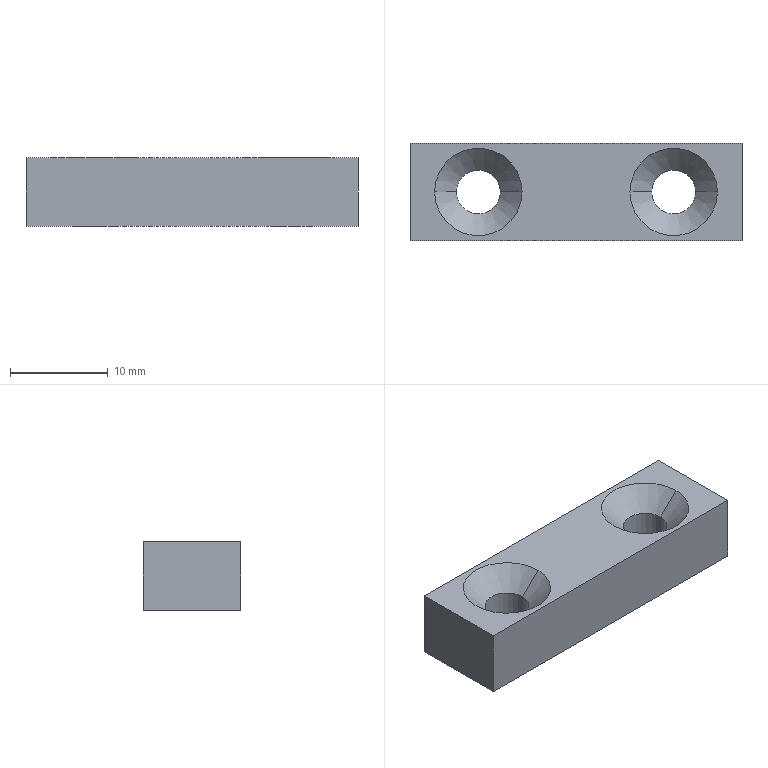Part | STEP file | anti-collision silicone pad | 1 solid | 14 faces | box 34 x 10 x 7 mm | volume 2064 mm3 | plane 6 | cone 4 | cylinder 4 | commonest cylinder face diameters 4.5 x4
STEP:
#1=CARTESIAN_POINT('',(0.,0.,0.));
#2=DIRECTION('',(0.,0.,1.));
#3=DIRECTION('',(1.,0.,0.));
#4=AXIS2_PLACEMENT_3D('',#1,#2,#3);
#5=CARTESIAN_POINT('',(-7.75,0.,4.77));
#6=VERTEX_POINT('',#5);
#7=CARTESIAN_POINT('',(-5.52,0.,7.));
#8=VERTEX_POINT('',#7);
#9=CARTESIAN_POINT('',(-5.52,0.,7.));
#10=DIRECTION('',(0.7071,0.,0.7071));
#11=VECTOR('',#10,1.);
#12=LINE('',#9,#11);
#13=CARTESIAN_POINT('',(-10.,0.,7.));
#14=DIRECTION('',(0.,0.,1.));
#15=DIRECTION('',(1.,0.,0.));
#16=AXIS2_PLACEMENT_3D('',#13,#14,#15);
#17=CONICAL_SURFACE('',#16,4.48,0.7854);
#18=CARTESIAN_POINT('',(6.283,0.));
#19=DIRECTION('',(0.,1.));
#20=VECTOR('',#19,1.);
#21=LINE('',#18,#20);
#22=(GEOMETRIC_REPRESENTATION_CONTEXT(2)PARAMETRIC_REPRESENTATION_CONTEXT()REPRESENTATION_CONTEXT('',''));
#23=DEFINITIONAL_REPRESENTATION('',(#21),#22);
#24=PCURVE('',#17,#23);
#25=CARTESIAN_POINT('',(-10.,0.,7.));
#26=DIRECTION('',(0.,0.,1.));
#27=DIRECTION('',(1.,0.,0.));
#28=AXIS2_PLACEMENT_3D('',#25,#26,#27);
#29=CONICAL_SURFACE('',#28,4.48,0.7854);
#30=CARTESIAN_POINT('',(0.,0.));
#31=DIRECTION('',(0.,1.));
#32=VECTOR('',#31,1.);
#33=LINE('',#30,#32);
#34=(GEOMETRIC_REPRESENTATION_CONTEXT(2)PARAMETRIC_REPRESENTATION_CONTEXT()REPRESENTATION_CONTEXT('',''));
#35=DEFINITIONAL_REPRESENTATION('',(#33),#34);
#36=PCURVE('',#29,#35);
#37=SURFACE_CURVE('',#12,(#24,#36),.PCURVE_S1.);
#38=EDGE_CURVE('',#6,#8,#37,.T.);
#39=ORIENTED_EDGE('',*,*,#38,.T.);
#40=CARTESIAN_POINT('',(-14.48,0.,7.));
#41=VERTEX_POINT('',#40);
#42=CARTESIAN_POINT('',(-10.,0.,7.));
#43=DIRECTION('',(0.,0.,1.));
#44=DIRECTION('',(1.,0.,0.));
#45=AXIS2_PLACEMENT_3D('',#42,#43,#44);
#46=CIRCLE('',#45,4.48);
#47=CARTESIAN_POINT('',(0.,0.));
#48=DIRECTION('',(1.,0.));
#49=VECTOR('',#48,1.);
#50=LINE('',#47,#49);
#51=(GEOMETRIC_REPRESENTATION_CONTEXT(2)PARAMETRIC_REPRESENTATION_CONTEXT()REPRESENTATION_CONTEXT('',''));
#52=DEFINITIONAL_REPRESENTATION('',(#50),#51);
#53=PCURVE('',#17,#52);
#54=CARTESIAN_POINT('',(-17.,5.,7.));
#55=DIRECTION('',(0.,0.,1.));
#56=DIRECTION('',(1.,0.,0.));
#57=AXIS2_PLACEMENT_3D('',#54,#55,#56);
#58=PLANE('',#57);
#59=CARTESIAN_POINT('',(7.,-5.));
#60=DIRECTION('',(1.,0.));
#61=AXIS2_PLACEMENT_2D('',#59,#60);
#62=CIRCLE('',#61,4.48);
#63=(GEOMETRIC_REPRESENTATION_CONTEXT(2)PARAMETRIC_REPRESENTATION_CONTEXT()REPRESENTATION_CONTEXT('',''));
#64=DEFINITIONAL_REPRESENTATION('',(#62),#63);
#65=PCURVE('',#58,#64);
#66=SURFACE_CURVE('',#46,(#53,#65),.PCURVE_S1.);
#67=EDGE_CURVE('',#41,#8,#66,.T.);
#68=ORIENTED_EDGE('',*,*,#67,.F.);
#69=CARTESIAN_POINT('',(-12.25,0.,4.77));
#70=VERTEX_POINT('',#69);
#71=CARTESIAN_POINT('',(-14.48,0.,7.));
#72=DIRECTION('',(-0.7071,0.,0.7071));
#73=VECTOR('',#72,1.);
#74=LINE('',#71,#73);
#75=CARTESIAN_POINT('',(3.142,0.));
#76=DIRECTION('',(0.,1.));
#77=VECTOR('',#76,1.);
#78=LINE('',#75,#77);
#79=(GEOMETRIC_REPRESENTATION_CONTEXT(2)PARAMETRIC_REPRESENTATION_CONTEXT()REPRESENTATION_CONTEXT('',''));
#80=DEFINITIONAL_REPRESENTATION('',(#78),#79);
#81=PCURVE('',#17,#80);
#82=CARTESIAN_POINT('',(3.142,0.));
#83=DIRECTION('',(0.,1.));
#84=VECTOR('',#83,1.);
#85=LINE('',#82,#84);
#86=(GEOMETRIC_REPRESENTATION_CONTEXT(2)PARAMETRIC_REPRESENTATION_CONTEXT()REPRESENTATION_CONTEXT('',''));
#87=DEFINITIONAL_REPRESENTATION('',(#85),#86);
#88=PCURVE('',#29,#87);
#89=SURFACE_CURVE('',#74,(#81,#88),.PCURVE_S1.);
#90=EDGE_CURVE('',#70,#41,#89,.T.);
#91=ORIENTED_EDGE('',*,*,#90,.F.);
#92=CARTESIAN_POINT('',(-10.,0.,4.77));
#93=DIRECTION('',(0.,0.,1.));
#94=DIRECTION('',(1.,0.,0.));
#95=AXIS2_PLACEMENT_3D('',#92,#93,#94);
#96=CIRCLE('',#95,2.25);
#97=CARTESIAN_POINT('',(0.,-2.23));
#98=DIRECTION('',(1.,0.));
#99=VECTOR('',#98,1.);
#100=LINE('',#97,#99);
#101=(GEOMETRIC_REPRESENTATION_CONTEXT(2)PARAMETRIC_REPRESENTATION_CONTEXT()REPRESENTATION_CONTEXT('',''));
#102=DEFINITIONAL_REPRESENTATION('',(#100),#101);
#103=PCURVE('',#17,#102);
#104=CARTESIAN_POINT('',(-10.,0.,7.));
#105=DIRECTION('',(0.,0.,1.));
#106=DIRECTION('',(1.,0.,0.));
#107=AXIS2_PLACEMENT_3D('',#104,#105,#106);
#108=CYLINDRICAL_SURFACE('',#107,2.25);
#109=CARTESIAN_POINT('',(0.,-2.23));
#110=DIRECTION('',(1.,0.));
#111=VECTOR('',#110,1.);
#112=LINE('',#109,#111);
#113=(GEOMETRIC_REPRESENTATION_CONTEXT(2)PARAMETRIC_REPRESENTATION_CONTEXT()REPRESENTATION_CONTEXT('',''));
#114=DEFINITIONAL_REPRESENTATION('',(#112),#113);
#115=PCURVE('',#108,#114);
#116=SURFACE_CURVE('',#96,(#103,#115),.PCURVE_S1.);
#117=EDGE_CURVE('',#70,#6,#116,.T.);
#118=ORIENTED_EDGE('',*,*,#117,.T.);
#119=EDGE_LOOP('',(#39,#68,#91,#118));
#120=FACE_BOUND('',#119,.F.);
#121=ADVANCED_FACE('',(#120),#17,.F.);
#122=CARTESIAN_POINT('',(-7.75,0.,0.));
#123=VERTEX_POINT('',#122);
#124=CARTESIAN_POINT('',(-7.75,0.,7.));
#125=DIRECTION('',(0.,0.,1.));
#126=VECTOR('',#125,1.);
#127=LINE('',#124,#126);
#128=CARTESIAN_POINT('',(6.283,0.));
#129=DIRECTION('',(0.,1.));
#130=VECTOR('',#129,1.);
#131=LINE('',#128,#130);
#132=(GEOMETRIC_REPRESENTATION_CONTEXT(2)PARAMETRIC_REPRESENTATION_CONTEXT()REPRESENTATION_CONTEXT('',''));
#133=DEFINITIONAL_REPRESENTATION('',(#131),#132);
#134=PCURVE('',#108,#133);
#135=CARTESIAN_POINT('',(-10.,0.,7.));
#136=DIRECTION('',(0.,0.,1.));
#137=DIRECTION('',(1.,0.,0.));
#138=AXIS2_PLACEMENT_3D('',#135,#136,#137);
#139=CYLINDRICAL_SURFACE('',#138,2.25);
#140=CARTESIAN_POINT('',(0.,0.));
#141=DIRECTION('',(0.,1.));
#142=VECTOR('',#141,1.);
#143=LINE('',#140,#142);
#144=(GEOMETRIC_REPRESENTATION_CONTEXT(2)PARAMETRIC_REPRESENTATION_CONTEXT()REPRESENTATION_CONTEXT('',''));
#145=DEFINITIONAL_REPRESENTATION('',(#143),#144);
#146=PCURVE('',#139,#145);
#147=SURFACE_CURVE('',#127,(#134,#146),.PCURVE_S1.);
#148=EDGE_CURVE('',#123,#6,#147,.T.);
#149=ORIENTED_EDGE('',*,*,#148,.T.);
#150=ORIENTED_EDGE('',*,*,#117,.F.);
#151=CARTESIAN_POINT('',(-12.25,0.,0.));
#152=VERTEX_POINT('',#151);
#153=CARTESIAN_POINT('',(-12.25,0.,7.));
#154=DIRECTION('',(0.,0.,1.));
#155=VECTOR('',#154,1.);
#156=LINE('',#153,#155);
#157=CARTESIAN_POINT('',(3.142,0.));
#158=DIRECTION('',(0.,1.));
#159=VECTOR('',#158,1.);
#160=LINE('',#157,#159);
#161=(GEOMETRIC_REPRESENTATION_CONTEXT(2)PARAMETRIC_REPRESENTATION_CONTEXT()REPRESENTATION_CONTEXT('',''));
#162=DEFINITIONAL_REPRESENTATION('',(#160),#161);
#163=PCURVE('',#108,#162);
#164=CARTESIAN_POINT('',(3.142,0.));
#165=DIRECTION('',(0.,1.));
#166=VECTOR('',#165,1.);
#167=LINE('',#164,#166);
#168=(GEOMETRIC_REPRESENTATION_CONTEXT(2)PARAMETRIC_REPRESENTATION_CONTEXT()REPRESENTATION_CONTEXT('',''));
#169=DEFINITIONAL_REPRESENTATION('',(#167),#168);
#170=PCURVE('',#139,#169);
#171=SURFACE_CURVE('',#156,(#163,#170),.PCURVE_S1.);
#172=EDGE_CURVE('',#152,#70,#171,.T.);
#173=ORIENTED_EDGE('',*,*,#172,.F.);
#174=CARTESIAN_POINT('',(-10.,0.,0.));
#175=DIRECTION('',(0.,0.,1.));
#176=DIRECTION('',(1.,0.,0.));
#177=AXIS2_PLACEMENT_3D('',#174,#175,#176);
#178=CIRCLE('',#177,2.25);
#179=CARTESIAN_POINT('',(0.,-7.));
#180=DIRECTION('',(1.,0.));
#181=VECTOR('',#180,1.);
#182=LINE('',#179,#181);
#183=(GEOMETRIC_REPRESENTATION_CONTEXT(2)PARAMETRIC_REPRESENTATION_CONTEXT()REPRESENTATION_CONTEXT('',''));
#184=DEFINITIONAL_REPRESENTATION('',(#182),#183);
#185=PCURVE('',#108,#184);
#186=CARTESIAN_POINT('',(-17.,5.,0.));
#187=DIRECTION('',(0.,0.,1.));
#188=DIRECTION('',(1.,0.,0.));
#189=AXIS2_PLACEMENT_3D('',#186,#187,#188);
#190=PLANE('',#189);
#191=CARTESIAN_POINT('',(7.,-5.));
#192=DIRECTION('',(1.,0.));
#193=AXIS2_PLACEMENT_2D('',#191,#192);
#194=CIRCLE('',#193,2.25);
#195=(GEOMETRIC_REPRESENTATION_CONTEXT(2)PARAMETRIC_REPRESENTATION_CONTEXT()REPRESENTATION_CONTEXT('',''));
#196=DEFINITIONAL_REPRESENTATION('',(#194),#195);
#197=PCURVE('',#190,#196);
#198=SURFACE_CURVE('',#178,(#185,#197),.PCURVE_S1.);
#199=EDGE_CURVE('',#152,#123,#198,.T.);
#200=ORIENTED_EDGE('',*,*,#199,.T.);
#201=EDGE_LOOP('',(#149,#150,#173,#200));
#202=FACE_BOUND('',#201,.F.);
#203=ADVANCED_FACE('',(#202),#108,.F.);
#204=CARTESIAN_POINT('',(12.25,0.,4.77));
#205=VERTEX_POINT('',#204);
#206=CARTESIAN_POINT('',(14.48,0.,7.));
#207=VERTEX_POINT('',#206);
#208=CARTESIAN_POINT('',(14.48,0.,7.));
#209=DIRECTION('',(0.7071,0.,0.7071));
#210=VECTOR('',#209,1.);
#211=LINE('',#208,#210);
#212=CARTESIAN_POINT('',(10.,0.,7.));
#213=DIRECTION('',(0.,0.,1.));
#214=DIRECTION('',(1.,0.,0.));
#215=AXIS2_PLACEMENT_3D('',#212,#213,#214);
#216=CONICAL_SURFACE('',#215,4.48,0.7854);
#217=CARTESIAN_POINT('',(6.283,0.));
#218=DIRECTION('',(0.,1.));
#219=VECTOR('',#218,1.);
#220=LINE('',#217,#219);
#221=(GEOMETRIC_REPRESENTATION_CONTEXT(2)PARAMETRIC_REPRESENTATION_CONTEXT()REPRESENTATION_CONTEXT('',''));
#222=DEFINITIONAL_REPRESENTATION('',(#220),#221);
#223=PCURVE('',#216,#222);
#224=CARTESIAN_POINT('',(10.,0.,7.));
#225=DIRECTION('',(0.,0.,1.));
#226=DIRECTION('',(1.,0.,0.));
#227=AXIS2_PLACEMENT_3D('',#224,#225,#226);
#228=CONICAL_SURFACE('',#227,4.48,0.7854);
#229=CARTESIAN_POINT('',(0.,0.));
#230=DIRECTION('',(0.,1.));
#231=VECTOR('',#230,1.);
#232=LINE('',#229,#231);
#233=(GEOMETRIC_REPRESENTATION_CONTEXT(2)PARAMETRIC_REPRESENTATION_CONTEXT()REPRESENTATION_CONTEXT('',''));
#234=DEFINITIONAL_REPRESENTATION('',(#232),#233);
#235=PCURVE('',#228,#234);
#236=SURFACE_CURVE('',#211,(#223,#235),.PCURVE_S1.);
#237=EDGE_CURVE('',#205,#207,#236,.T.);
#238=ORIENTED_EDGE('',*,*,#237,.T.);
#239=CARTESIAN_POINT('',(5.52,0.,7.));
#240=VERTEX_POINT('',#239);
#241=CARTESIAN_POINT('',(10.,0.,7.));
#242=DIRECTION('',(0.,0.,1.));
#243=DIRECTION('',(1.,0.,0.));
#244=AXIS2_PLACEMENT_3D('',#241,#242,#243);
#245=CIRCLE('',#244,4.48);
#246=CARTESIAN_POINT('',(0.,0.));
#247=DIRECTION('',(1.,0.));
#248=VECTOR('',#247,1.);
#249=LINE('',#246,#248);
#250=(GEOMETRIC_REPRESENTATION_CONTEXT(2)PARAMETRIC_REPRESENTATION_CONTEXT()REPRESENTATION_CONTEXT('',''));
#251=DEFINITIONAL_REPRESENTATION('',(#249),#250);
#252=PCURVE('',#216,#251);
#253=CARTESIAN_POINT('',(27.,-5.));
#254=DIRECTION('',(1.,0.));
#255=AXIS2_PLACEMENT_2D('',#253,#254);
#256=CIRCLE('',#255,4.48);
#257=(GEOMETRIC_REPRESENTATION_CONTEXT(2)PARAMETRIC_REPRESENTATION_CONTEXT()REPRESENTATION_CONTEXT('',''));
#258=DEFINITIONAL_REPRESENTATION('',(#256),#257);
#259=PCURVE('',#58,#258);
#260=SURFACE_CURVE('',#245,(#252,#259),.PCURVE_S1.);
#261=EDGE_CURVE('',#240,#207,#260,.T.);
#262=ORIENTED_EDGE('',*,*,#261,.F.);
#263=CARTESIAN_POINT('',(7.75,0.,4.77));
#264=VERTEX_POINT('',#263);
#265=CARTESIAN_POINT('',(5.52,0.,7.));
#266=DIRECTION('',(-0.7071,0.,0.7071));
#267=VECTOR('',#266,1.);
#268=LINE('',#265,#267);
#269=CARTESIAN_POINT('',(3.142,0.));
#270=DIRECTION('',(0.,1.));
#271=VECTOR('',#270,1.);
#272=LINE('',#269,#271);
#273=(GEOMETRIC_REPRESENTATION_CONTEXT(2)PARAMETRIC_REPRESENTATION_CONTEXT()REPRESENTATION_CONTEXT('',''));
#274=DEFINITIONAL_REPRESENTATION('',(#272),#273);
#275=PCURVE('',#216,#274);
#276=CARTESIAN_POINT('',(3.142,0.));
#277=DIRECTION('',(0.,1.));
#278=VECTOR('',#277,1.);
#279=LINE('',#276,#278);
#280=(GEOMETRIC_REPRESENTATION_CONTEXT(2)PARAMETRIC_REPRESENTATION_CONTEXT()REPRESENTATION_CONTEXT('',''));
#281=DEFINITIONAL_REPRESENTATION('',(#279),#280);
#282=PCURVE('',#228,#281);
#283=SURFACE_CURVE('',#268,(#275,#282),.PCURVE_S1.);
#284=EDGE_CURVE('',#264,#240,#283,.T.);
#285=ORIENTED_EDGE('',*,*,#284,.F.);
#286=CARTESIAN_POINT('',(10.,0.,4.77));
#287=DIRECTION('',(0.,0.,1.));
#288=DIRECTION('',(1.,0.,0.));
#289=AXIS2_PLACEMENT_3D('',#286,#287,#288);
#290=CIRCLE('',#289,2.25);
#291=CARTESIAN_POINT('',(0.,-2.23));
#292=DIRECTION('',(1.,0.));
#293=VECTOR('',#292,1.);
#294=LINE('',#291,#293);
#295=(GEOMETRIC_REPRESENTATION_CONTEXT(2)PARAMETRIC_REPRESENTATION_CONTEXT()REPRESENTATION_CONTEXT('',''));
#296=DEFINITIONAL_REPRESENTATION('',(#294),#295);
#297=PCURVE('',#216,#296);
#298=CARTESIAN_POINT('',(10.,0.,7.));
#299=DIRECTION('',(0.,0.,1.));
#300=DIRECTION('',(1.,0.,0.));
#301=AXIS2_PLACEMENT_3D('',#298,#299,#300);
#302=CYLINDRICAL_SURFACE('',#301,2.25);
#303=CARTESIAN_POINT('',(0.,-2.23));
#304=DIRECTION('',(1.,0.));
#305=VECTOR('',#304,1.);
#306=LINE('',#303,#305);
#307=(GEOMETRIC_REPRESENTATION_CONTEXT(2)PARAMETRIC_REPRESENTATION_CONTEXT()REPRESENTATION_CONTEXT('',''));
#308=DEFINITIONAL_REPRESENTATION('',(#306),#307);
#309=PCURVE('',#302,#308);
#310=SURFACE_CURVE('',#290,(#297,#309),.PCURVE_S1.);
#311=EDGE_CURVE('',#264,#205,#310,.T.);
#312=ORIENTED_EDGE('',*,*,#311,.T.);
#313=EDGE_LOOP('',(#238,#262,#285,#312));
#314=FACE_BOUND('',#313,.F.);
#315=ADVANCED_FACE('',(#314),#216,.F.);
#316=CARTESIAN_POINT('',(12.25,0.,0.));
#317=VERTEX_POINT('',#316);
#318=CARTESIAN_POINT('',(12.25,0.,7.));
#319=DIRECTION('',(0.,0.,1.));
#320=VECTOR('',#319,1.);
#321=LINE('',#318,#320);
#322=CARTESIAN_POINT('',(6.283,0.));
#323=DIRECTION('',(0.,1.));
#324=VECTOR('',#323,1.);
#325=LINE('',#322,#324);
#326=(GEOMETRIC_REPRESENTATION_CONTEXT(2)PARAMETRIC_REPRESENTATION_CONTEXT()REPRESENTATION_CONTEXT('',''));
#327=DEFINITIONAL_REPRESENTATION('',(#325),#326);
#328=PCURVE('',#302,#327);
#329=CARTESIAN_POINT('',(10.,0.,7.));
#330=DIRECTION('',(0.,0.,1.));
#331=DIRECTION('',(1.,0.,0.));
#332=AXIS2_PLACEMENT_3D('',#329,#330,#331);
#333=CYLINDRICAL_SURFACE('',#332,2.25);
#334=CARTESIAN_POINT('',(0.,0.));
#335=DIRECTION('',(0.,1.));
#336=VECTOR('',#335,1.);
#337=LINE('',#334,#336);
#338=(GEOMETRIC_REPRESENTATION_CONTEXT(2)PARAMETRIC_REPRESENTATION_CONTEXT()REPRESENTATION_CONTEXT('',''));
#339=DEFINITIONAL_REPRESENTATION('',(#337),#338);
#340=PCURVE('',#333,#339);
#341=SURFACE_CURVE('',#321,(#328,#340),.PCURVE_S1.);
#342=EDGE_CURVE('',#317,#205,#341,.T.);
#343=ORIENTED_EDGE('',*,*,#342,.T.);
#344=ORIENTED_EDGE('',*,*,#311,.F.);
#345=CARTESIAN_POINT('',(7.75,0.,0.));
#346=VERTEX_POINT('',#345);
#347=CARTESIAN_POINT('',(7.75,0.,7.));
#348=DIRECTION('',(0.,0.,1.));
#349=VECTOR('',#348,1.);
#350=LINE('',#347,#349);
#351=CARTESIAN_POINT('',(3.142,0.));
#352=DIRECTION('',(0.,1.));
#353=VECTOR('',#352,1.);
#354=LINE('',#351,#353);
#355=(GEOMETRIC_REPRESENTATION_CONTEXT(2)PARAMETRIC_REPRESENTATION_CONTEXT()REPRESENTATION_CONTEXT('',''));
#356=DEFINITIONAL_REPRESENTATION('',(#354),#355);
#357=PCURVE('',#302,#356);
#358=CARTESIAN_POINT('',(3.142,0.));
#359=DIRECTION('',(0.,1.));
#360=VECTOR('',#359,1.);
#361=LINE('',#358,#360);
#362=(GEOMETRIC_REPRESENTATION_CONTEXT(2)PARAMETRIC_REPRESENTATION_CONTEXT()REPRESENTATION_CONTEXT('',''));
#363=DEFINITIONAL_REPRESENTATION('',(#361),#362);
#364=PCURVE('',#333,#363);
#365=SURFACE_CURVE('',#350,(#357,#364),.PCURVE_S1.);
#366=EDGE_CURVE('',#346,#264,#365,.T.);
#367=ORIENTED_EDGE('',*,*,#366,.F.);
#368=CARTESIAN_POINT('',(10.,0.,0.));
#369=DIRECTION('',(0.,0.,1.));
#370=DIRECTION('',(1.,0.,0.));
#371=AXIS2_PLACEMENT_3D('',#368,#369,#370);
#372=CIRCLE('',#371,2.25);
#373=CARTESIAN_POINT('',(0.,-7.));
#374=DIRECTION('',(1.,0.));
#375=VECTOR('',#374,1.);
#376=LINE('',#373,#375);
#377=(GEOMETRIC_REPRESENTATION_CONTEXT(2)PARAMETRIC_REPRESENTATION_CONTEXT()REPRESENTATION_CONTEXT('',''));
#378=DEFINITIONAL_REPRESENTATION('',(#376),#377);
#379=PCURVE('',#302,#378);
#380=CARTESIAN_POINT('',(27.,-5.));
#381=DIRECTION('',(1.,0.));
#382=AXIS2_PLACEMENT_2D('',#380,#381);
#383=CIRCLE('',#382,2.25);
#384=(GEOMETRIC_REPRESENTATION_CONTEXT(2)PARAMETRIC_REPRESENTATION_CONTEXT()REPRESENTATION_CONTEXT('',''));
#385=DEFINITIONAL_REPRESENTATION('',(#383),#384);
#386=PCURVE('',#190,#385);
#387=SURFACE_CURVE('',#372,(#379,#386),.PCURVE_S1.);
#388=EDGE_CURVE('',#346,#317,#387,.T.);
#389=ORIENTED_EDGE('',*,*,#388,.T.);
#390=EDGE_LOOP('',(#343,#344,#367,#389));
#391=FACE_BOUND('',#390,.F.);
#392=ADVANCED_FACE('',(#391),#302,.F.);
#393=CARTESIAN_POINT('',(-17.,5.,0.));
#394=VERTEX_POINT('',#393);
#395=CARTESIAN_POINT('',(-17.,-5.,0.));
#396=VERTEX_POINT('',#395);
#397=CARTESIAN_POINT('',(-17.,-5.,0.));
#398=DIRECTION('',(0.,-1.,0.));
#399=VECTOR('',#398,1.);
#400=LINE('',#397,#399);
#401=CARTESIAN_POINT('',(-17.,-5.,7.));
#402=DIRECTION('',(1.,0.,0.));
#403=DIRECTION('',(0.,0.,-1.));
#404=AXIS2_PLACEMENT_3D('',#401,#402,#403);
#405=PLANE('',#404);
#406=CARTESIAN_POINT('',(7.,0.));
#407=DIRECTION('',(0.,-1.));
#408=VECTOR('',#407,1.);
#409=LINE('',#406,#408);
#410=(GEOMETRIC_REPRESENTATION_CONTEXT(2)PARAMETRIC_REPRESENTATION_CONTEXT()REPRESENTATION_CONTEXT('',''));
#411=DEFINITIONAL_REPRESENTATION('',(#409),#410);
#412=PCURVE('',#405,#411);
#413=CARTESIAN_POINT('',(0.,-10.));
#414=DIRECTION('',(0.,-1.));
#415=VECTOR('',#414,1.);
#416=LINE('',#413,#415);
#417=(GEOMETRIC_REPRESENTATION_CONTEXT(2)PARAMETRIC_REPRESENTATION_CONTEXT()REPRESENTATION_CONTEXT('',''));
#418=DEFINITIONAL_REPRESENTATION('',(#416),#417);
#419=PCURVE('',#190,#418);
#420=SURFACE_CURVE('',#400,(#412,#419),.PCURVE_S1.);
#421=EDGE_CURVE('',#394,#396,#420,.T.);
#422=ORIENTED_EDGE('',*,*,#421,.T.);
#423=CARTESIAN_POINT('',(-17.,-5.,7.));
#424=VERTEX_POINT('',#423);
#425=CARTESIAN_POINT('',(-17.,-5.,7.));
#426=DIRECTION('',(0.,0.,-1.));
#427=VECTOR('',#426,1.);
#428=LINE('',#425,#427);
#429=CARTESIAN_POINT('',(0.,0.));
#430=DIRECTION('',(1.,0.));
#431=VECTOR('',#430,1.);
#432=LINE('',#429,#431);
#433=(GEOMETRIC_REPRESENTATION_CONTEXT(2)PARAMETRIC_REPRESENTATION_CONTEXT()REPRESENTATION_CONTEXT('',''));
#434=DEFINITIONAL_REPRESENTATION('',(#432),#433);
#435=PCURVE('',#405,#434);
#436=CARTESIAN_POINT('',(17.,-5.,7.));
#437=DIRECTION('',(0.,1.,0.));
#438=DIRECTION('',(-1.,0.,0.));
#439=AXIS2_PLACEMENT_3D('',#436,#437,#438);
#440=PLANE('',#439);
#441=CARTESIAN_POINT('',(34.,0.));
#442=DIRECTION('',(0.,-1.));
#443=VECTOR('',#442,1.);
#444=LINE('',#441,#443);
#445=(GEOMETRIC_REPRESENTATION_CONTEXT(2)PARAMETRIC_REPRESENTATION_CONTEXT()REPRESENTATION_CONTEXT('',''));
#446=DEFINITIONAL_REPRESENTATION('',(#444),#445);
#447=PCURVE('',#440,#446);
#448=SURFACE_CURVE('',#428,(#435,#447),.PCURVE_S1.);
#449=EDGE_CURVE('',#424,#396,#448,.T.);
#450=ORIENTED_EDGE('',*,*,#449,.F.);
#451=CARTESIAN_POINT('',(-17.,5.,7.));
#452=VERTEX_POINT('',#451);
#453=CARTESIAN_POINT('',(-17.,-5.,7.));
#454=DIRECTION('',(0.,-1.,0.));
#455=VECTOR('',#454,1.);
#456=LINE('',#453,#455);
#457=CARTESIAN_POINT('',(0.,0.));
#458=DIRECTION('',(0.,-1.));
#459=VECTOR('',#458,1.);
#460=LINE('',#457,#459);
#461=(GEOMETRIC_REPRESENTATION_CONTEXT(2)PARAMETRIC_REPRESENTATION_CONTEXT()REPRESENTATION_CONTEXT('',''));
#462=DEFINITIONAL_REPRESENTATION('',(#460),#461);
#463=PCURVE('',#405,#462);
#464=CARTESIAN_POINT('',(0.,-10.));
#465=DIRECTION('',(0.,-1.));
#466=VECTOR('',#465,1.);
#467=LINE('',#464,#466);
#468=(GEOMETRIC_REPRESENTATION_CONTEXT(2)PARAMETRIC_REPRESENTATION_CONTEXT()REPRESENTATION_CONTEXT('',''));
#469=DEFINITIONAL_REPRESENTATION('',(#467),#468);
#470=PCURVE('',#58,#469);
#471=SURFACE_CURVE('',#456,(#463,#470),.PCURVE_S1.);
#472=EDGE_CURVE('',#452,#424,#471,.T.);
#473=ORIENTED_EDGE('',*,*,#472,.F.);
#474=CARTESIAN_POINT('',(-17.,5.,7.));
#475=DIRECTION('',(0.,0.,-1.));
#476=VECTOR('',#475,1.);
#477=LINE('',#474,#476);
#478=CARTESIAN_POINT('',(0.,10.));
#479=DIRECTION('',(1.,0.));
#480=VECTOR('',#479,1.);
#481=LINE('',#478,#480);
#482=(GEOMETRIC_REPRESENTATION_CONTEXT(2)PARAMETRIC_REPRESENTATION_CONTEXT()REPRESENTATION_CONTEXT('',''));
#483=DEFINITIONAL_REPRESENTATION('',(#481),#482);
#484=PCURVE('',#405,#483);
#485=CARTESIAN_POINT('',(17.,5.,7.));
#486=DIRECTION('',(0.,-1.,0.));
#487=DIRECTION('',(1.,0.,0.));
#488=AXIS2_PLACEMENT_3D('',#485,#486,#487);
#489=PLANE('',#488);
#490=CARTESIAN_POINT('',(-34.,0.));
#491=DIRECTION('',(0.,-1.));
#492=VECTOR('',#491,1.);
#493=LINE('',#490,#492);
#494=(GEOMETRIC_REPRESENTATION_CONTEXT(2)PARAMETRIC_REPRESENTATION_CONTEXT()REPRESENTATION_CONTEXT('',''));
#495=DEFINITIONAL_REPRESENTATION('',(#493),#494);
#496=PCURVE('',#489,#495);
#497=SURFACE_CURVE('',#477,(#484,#496),.PCURVE_S1.);
#498=EDGE_CURVE('',#452,#394,#497,.T.);
#499=ORIENTED_EDGE('',*,*,#498,.T.);
#500=EDGE_LOOP('',(#422,#450,#473,#499));
#501=FACE_BOUND('',#500,.T.);
#502=ADVANCED_FACE('',(#501),#405,.F.);
#503=CARTESIAN_POINT('',(17.,-5.,0.));
#504=VERTEX_POINT('',#503);
#505=CARTESIAN_POINT('',(17.,-5.,0.));
#506=DIRECTION('',(1.,0.,0.));
#507=VECTOR('',#506,1.);
#508=LINE('',#505,#507);
#509=CARTESIAN_POINT('',(0.,-7.));
#510=DIRECTION('',(-1.,0.));
#511=VECTOR('',#510,1.);
#512=LINE('',#509,#511);
#513=(GEOMETRIC_REPRESENTATION_CONTEXT(2)PARAMETRIC_REPRESENTATION_CONTEXT()REPRESENTATION_CONTEXT('',''));
#514=DEFINITIONAL_REPRESENTATION('',(#512),#513);
#515=PCURVE('',#440,#514);
#516=CARTESIAN_POINT('',(34.,-10.));
#517=DIRECTION('',(1.,0.));
#518=VECTOR('',#517,1.);
#519=LINE('',#516,#518);
#520=(GEOMETRIC_REPRESENTATION_CONTEXT(2)PARAMETRIC_REPRESENTATION_CONTEXT()REPRESENTATION_CONTEXT('',''));
#521=DEFINITIONAL_REPRESENTATION('',(#519),#520);
#522=PCURVE('',#190,#521);
#523=SURFACE_CURVE('',#508,(#515,#522),.PCURVE_S1.);
#524=EDGE_CURVE('',#396,#504,#523,.T.);
#525=ORIENTED_EDGE('',*,*,#524,.T.);
#526=CARTESIAN_POINT('',(17.,-5.,7.));
#527=VERTEX_POINT('',#526);
#528=CARTESIAN_POINT('',(17.,-5.,7.));
#529=DIRECTION('',(0.,0.,-1.));
#530=VECTOR('',#529,1.);
#531=LINE('',#528,#530);
#532=CARTESIAN_POINT('',(0.,0.));
#533=DIRECTION('',(0.,-1.));
#534=VECTOR('',#533,1.);
#535=LINE('',#532,#534);
#536=(GEOMETRIC_REPRESENTATION_CONTEXT(2)PARAMETRIC_REPRESENTATION_CONTEXT()REPRESENTATION_CONTEXT('',''));
#537=DEFINITIONAL_REPRESENTATION('',(#535),#536);
#538=PCURVE('',#440,#537);
#539=CARTESIAN_POINT('',(17.,-5.,7.));
#540=DIRECTION('',(-1.,0.,0.));
#541=DIRECTION('',(0.,0.,1.));
#542=AXIS2_PLACEMENT_3D('',#539,#540,#541);
#543=PLANE('',#542);
#544=CARTESIAN_POINT('',(0.,0.));
#545=DIRECTION('',(-1.,0.));
#546=VECTOR('',#545,1.);
#547=LINE('',#544,#546);
#548=(GEOMETRIC_REPRESENTATION_CONTEXT(2)PARAMETRIC_REPRESENTATION_CONTEXT()REPRESENTATION_CONTEXT('',''));
#549=DEFINITIONAL_REPRESENTATION('',(#547),#548);
#550=PCURVE('',#543,#549);
#551=SURFACE_CURVE('',#531,(#538,#550),.PCURVE_S1.);
#552=EDGE_CURVE('',#527,#504,#551,.T.);
#553=ORIENTED_EDGE('',*,*,#552,.F.);
#554=CARTESIAN_POINT('',(17.,-5.,7.));
#555=DIRECTION('',(1.,0.,0.));
#556=VECTOR('',#555,1.);
#557=LINE('',#554,#556);
#558=CARTESIAN_POINT('',(0.,0.));
#559=DIRECTION('',(-1.,0.));
#560=VECTOR('',#559,1.);
#561=LINE('',#558,#560);
#562=(GEOMETRIC_REPRESENTATION_CONTEXT(2)PARAMETRIC_REPRESENTATION_CONTEXT()REPRESENTATION_CONTEXT('',''));
#563=DEFINITIONAL_REPRESENTATION('',(#561),#562);
#564=PCURVE('',#440,#563);
#565=CARTESIAN_POINT('',(34.,-10.));
#566=DIRECTION('',(1.,0.));
#567=VECTOR('',#566,1.);
#568=LINE('',#565,#567);
#569=(GEOMETRIC_REPRESENTATION_CONTEXT(2)PARAMETRIC_REPRESENTATION_CONTEXT()REPRESENTATION_CONTEXT('',''));
#570=DEFINITIONAL_REPRESENTATION('',(#568),#569);
#571=PCURVE('',#58,#570);
#572=SURFACE_CURVE('',#557,(#564,#571),.PCURVE_S1.);
#573=EDGE_CURVE('',#424,#527,#572,.T.);
#574=ORIENTED_EDGE('',*,*,#573,.F.);
#575=ORIENTED_EDGE('',*,*,#449,.T.);
#576=EDGE_LOOP('',(#525,#553,#574,#575));
#577=FACE_BOUND('',#576,.T.);
#578=ADVANCED_FACE('',(#577),#440,.F.);
#579=CARTESIAN_POINT('',(17.,5.,0.));
#580=VERTEX_POINT('',#579);
#581=CARTESIAN_POINT('',(17.,-5.,0.));
#582=DIRECTION('',(0.,1.,0.));
#583=VECTOR('',#582,1.);
#584=LINE('',#581,#583);
#585=CARTESIAN_POINT('',(-7.,0.));
#586=DIRECTION('',(0.,1.));
#587=VECTOR('',#586,1.);
#588=LINE('',#585,#587);
#589=(GEOMETRIC_REPRESENTATION_CONTEXT(2)PARAMETRIC_REPRESENTATION_CONTEXT()REPRESENTATION_CONTEXT('',''));
#590=DEFINITIONAL_REPRESENTATION('',(#588),#589);
#591=PCURVE('',#543,#590);
#592=CARTESIAN_POINT('',(34.,-10.));
#593=DIRECTION('',(0.,1.));
#594=VECTOR('',#593,1.);
#595=LINE('',#592,#594);
#596=(GEOMETRIC_REPRESENTATION_CONTEXT(2)PARAMETRIC_REPRESENTATION_CONTEXT()REPRESENTATION_CONTEXT('',''));
#597=DEFINITIONAL_REPRESENTATION('',(#595),#596);
#598=PCURVE('',#190,#597);
#599=SURFACE_CURVE('',#584,(#591,#598),.PCURVE_S1.);
#600=EDGE_CURVE('',#504,#580,#599,.T.);
#601=ORIENTED_EDGE('',*,*,#600,.T.);
#602=CARTESIAN_POINT('',(17.,5.,7.));
#603=VERTEX_POINT('',#602);
#604=CARTESIAN_POINT('',(17.,5.,7.));
#605=DIRECTION('',(0.,0.,-1.));
#606=VECTOR('',#605,1.);
#607=LINE('',#604,#606);
#608=CARTESIAN_POINT('',(0.,10.));
#609=DIRECTION('',(-1.,0.));
#610=VECTOR('',#609,1.);
#611=LINE('',#608,#610);
#612=(GEOMETRIC_REPRESENTATION_CONTEXT(2)PARAMETRIC_REPRESENTATION_CONTEXT()REPRESENTATION_CONTEXT('',''));
#613=DEFINITIONAL_REPRESENTATION('',(#611),#612);
#614=PCURVE('',#543,#613);
#615=CARTESIAN_POINT('',(0.,0.));
#616=DIRECTION('',(0.,-1.));
#617=VECTOR('',#616,1.);
#618=LINE('',#615,#617);
#619=(GEOMETRIC_REPRESENTATION_CONTEXT(2)PARAMETRIC_REPRESENTATION_CONTEXT()REPRESENTATION_CONTEXT('',''));
#620=DEFINITIONAL_REPRESENTATION('',(#618),#619);
#621=PCURVE('',#489,#620);
#622=SURFACE_CURVE('',#607,(#614,#621),.PCURVE_S1.);
#623=EDGE_CURVE('',#603,#580,#622,.T.);
#624=ORIENTED_EDGE('',*,*,#623,.F.);
#625=CARTESIAN_POINT('',(17.,-5.,7.));
#626=DIRECTION('',(0.,1.,0.));
#627=VECTOR('',#626,1.);
#628=LINE('',#625,#627);
#629=CARTESIAN_POINT('',(0.,0.));
#630=DIRECTION('',(0.,1.));
#631=VECTOR('',#630,1.);
#632=LINE('',#629,#631);
#633=(GEOMETRIC_REPRESENTATION_CONTEXT(2)PARAMETRIC_REPRESENTATION_CONTEXT()REPRESENTATION_CONTEXT('',''));
#634=DEFINITIONAL_REPRESENTATION('',(#632),#633);
#635=PCURVE('',#543,#634);
#636=CARTESIAN_POINT('',(34.,-10.));
#637=DIRECTION('',(0.,1.));
#638=VECTOR('',#637,1.);
#639=LINE('',#636,#638);
#640=(GEOMETRIC_REPRESENTATION_CONTEXT(2)PARAMETRIC_REPRESENTATION_CONTEXT()REPRESENTATION_CONTEXT('',''));
#641=DEFINITIONAL_REPRESENTATION('',(#639),#640);
#642=PCURVE('',#58,#641);
#643=SURFACE_CURVE('',#628,(#635,#642),.PCURVE_S1.);
#644=EDGE_CURVE('',#527,#603,#643,.T.);
#645=ORIENTED_EDGE('',*,*,#644,.F.);
#646=ORIENTED_EDGE('',*,*,#552,.T.);
#647=EDGE_LOOP('',(#601,#624,#645,#646));
#648=FACE_BOUND('',#647,.T.);
#649=ADVANCED_FACE('',(#648),#543,.F.);
#650=CARTESIAN_POINT('',(17.,5.,0.));
#651=DIRECTION('',(-1.,0.,0.));
#652=VECTOR('',#651,1.);
#653=LINE('',#650,#652);
#654=CARTESIAN_POINT('',(0.,-7.));
#655=DIRECTION('',(-1.,0.));
#656=VECTOR('',#655,1.);
#657=LINE('',#654,#656);
#658=(GEOMETRIC_REPRESENTATION_CONTEXT(2)PARAMETRIC_REPRESENTATION_CONTEXT()REPRESENTATION_CONTEXT('',''));
#659=DEFINITIONAL_REPRESENTATION('',(#657),#658);
#660=PCURVE('',#489,#659);
#661=CARTESIAN_POINT('',(34.,0.));
#662=DIRECTION('',(-1.,0.));
#663=VECTOR('',#662,1.);
#664=LINE('',#661,#663);
#665=(GEOMETRIC_REPRESENTATION_CONTEXT(2)PARAMETRIC_REPRESENTATION_CONTEXT()REPRESENTATION_CONTEXT('',''));
#666=DEFINITIONAL_REPRESENTATION('',(#664),#665);
#667=PCURVE('',#190,#666);
#668=SURFACE_CURVE('',#653,(#660,#667),.PCURVE_S1.);
#669=EDGE_CURVE('',#580,#394,#668,.T.);
#670=ORIENTED_EDGE('',*,*,#669,.T.);
#671=ORIENTED_EDGE('',*,*,#498,.F.);
#672=CARTESIAN_POINT('',(17.,5.,7.));
#673=DIRECTION('',(-1.,0.,0.));
#674=VECTOR('',#673,1.);
#675=LINE('',#672,#674);
#676=CARTESIAN_POINT('',(0.,0.));
#677=DIRECTION('',(-1.,0.));
#678=VECTOR('',#677,1.);
#679=LINE('',#676,#678);
#680=(GEOMETRIC_REPRESENTATION_CONTEXT(2)PARAMETRIC_REPRESENTATION_CONTEXT()REPRESENTATION_CONTEXT('',''));
#681=DEFINITIONAL_REPRESENTATION('',(#679),#680);
#682=PCURVE('',#489,#681);
#683=CARTESIAN_POINT('',(34.,0.));
#684=DIRECTION('',(-1.,0.));
#685=VECTOR('',#684,1.);
#686=LINE('',#683,#685);
#687=(GEOMETRIC_REPRESENTATION_CONTEXT(2)PARAMETRIC_REPRESENTATION_CONTEXT()REPRESENTATION_CONTEXT('',''));
#688=DEFINITIONAL_REPRESENTATION('',(#686),#687);
#689=PCURVE('',#58,#688);
#690=SURFACE_CURVE('',#675,(#682,#689),.PCURVE_S1.);
#691=EDGE_CURVE('',#603,#452,#690,.T.);
#692=ORIENTED_EDGE('',*,*,#691,.F.);
#693=ORIENTED_EDGE('',*,*,#623,.T.);
#694=EDGE_LOOP('',(#670,#671,#692,#693));
#695=FACE_BOUND('',#694,.T.);
#696=ADVANCED_FACE('',(#695),#489,.F.);
#697=CARTESIAN_POINT('',(-10.,0.,7.));
#698=DIRECTION('',(0.,0.,1.));
#699=DIRECTION('',(1.,0.,0.));
#700=AXIS2_PLACEMENT_3D('',#697,#698,#699);
#701=CIRCLE('',#700,4.48);
#702=CARTESIAN_POINT('',(7.,-5.));
#703=DIRECTION('',(1.,0.));
#704=AXIS2_PLACEMENT_2D('',#702,#703);
#705=CIRCLE('',#704,4.48);
#706=(GEOMETRIC_REPRESENTATION_CONTEXT(2)PARAMETRIC_REPRESENTATION_CONTEXT()REPRESENTATION_CONTEXT('',''));
#707=DEFINITIONAL_REPRESENTATION('',(#705),#706);
#708=PCURVE('',#58,#707);
#709=CARTESIAN_POINT('',(0.,0.));
#710=DIRECTION('',(1.,0.));
#711=VECTOR('',#710,1.);
#712=LINE('',#709,#711);
#713=(GEOMETRIC_REPRESENTATION_CONTEXT(2)PARAMETRIC_REPRESENTATION_CONTEXT()REPRESENTATION_CONTEXT('',''));
#714=DEFINITIONAL_REPRESENTATION('',(#712),#713);
#715=PCURVE('',#29,#714);
#716=SURFACE_CURVE('',#701,(#708,#715),.PCURVE_S1.);
#717=EDGE_CURVE('',#8,#41,#716,.T.);
#718=ORIENTED_EDGE('',*,*,#717,.F.);
#719=ORIENTED_EDGE('',*,*,#67,.F.);
#720=EDGE_LOOP('',(#718,#719));
#721=FACE_BOUND('',#720,.T.);
#722=CARTESIAN_POINT('',(10.,0.,7.));
#723=DIRECTION('',(0.,0.,1.));
#724=DIRECTION('',(1.,0.,0.));
#725=AXIS2_PLACEMENT_3D('',#722,#723,#724);
#726=CIRCLE('',#725,4.48);
#727=CARTESIAN_POINT('',(27.,-5.));
#728=DIRECTION('',(1.,0.));
#729=AXIS2_PLACEMENT_2D('',#727,#728);
#730=CIRCLE('',#729,4.48);
#731=(GEOMETRIC_REPRESENTATION_CONTEXT(2)PARAMETRIC_REPRESENTATION_CONTEXT()REPRESENTATION_CONTEXT('',''));
#732=DEFINITIONAL_REPRESENTATION('',(#730),#731);
#733=PCURVE('',#58,#732);
#734=CARTESIAN_POINT('',(0.,0.));
#735=DIRECTION('',(1.,0.));
#736=VECTOR('',#735,1.);
#737=LINE('',#734,#736);
#738=(GEOMETRIC_REPRESENTATION_CONTEXT(2)PARAMETRIC_REPRESENTATION_CONTEXT()REPRESENTATION_CONTEXT('',''));
#739=DEFINITIONAL_REPRESENTATION('',(#737),#738);
#740=PCURVE('',#228,#739);
#741=SURFACE_CURVE('',#726,(#733,#740),.PCURVE_S1.);
#742=EDGE_CURVE('',#207,#240,#741,.T.);
#743=ORIENTED_EDGE('',*,*,#742,.F.);
#744=ORIENTED_EDGE('',*,*,#261,.F.);
#745=EDGE_LOOP('',(#743,#744));
#746=FACE_BOUND('',#745,.T.);
#747=ORIENTED_EDGE('',*,*,#472,.T.);
#748=ORIENTED_EDGE('',*,*,#573,.T.);
#749=ORIENTED_EDGE('',*,*,#644,.T.);
#750=ORIENTED_EDGE('',*,*,#691,.T.);
#751=EDGE_LOOP('',(#747,#748,#749,#750));
#752=FACE_BOUND('',#751,.T.);
#753=ADVANCED_FACE('',(#721,#746,#752),#58,.T.);
#754=CARTESIAN_POINT('',(-10.,0.,0.));
#755=DIRECTION('',(0.,0.,1.));
#756=DIRECTION('',(1.,0.,0.));
#757=AXIS2_PLACEMENT_3D('',#754,#755,#756);
#758=CIRCLE('',#757,2.25);
#759=CARTESIAN_POINT('',(7.,-5.));
#760=DIRECTION('',(1.,0.));
#761=AXIS2_PLACEMENT_2D('',#759,#760);
#762=CIRCLE('',#761,2.25);
#763=(GEOMETRIC_REPRESENTATION_CONTEXT(2)PARAMETRIC_REPRESENTATION_CONTEXT()REPRESENTATION_CONTEXT('',''));
#764=DEFINITIONAL_REPRESENTATION('',(#762),#763);
#765=PCURVE('',#190,#764);
#766=CARTESIAN_POINT('',(0.,-7.));
#767=DIRECTION('',(1.,0.));
#768=VECTOR('',#767,1.);
#769=LINE('',#766,#768);
#770=(GEOMETRIC_REPRESENTATION_CONTEXT(2)PARAMETRIC_REPRESENTATION_CONTEXT()REPRESENTATION_CONTEXT('',''));
#771=DEFINITIONAL_REPRESENTATION('',(#769),#770);
#772=PCURVE('',#139,#771);
#773=SURFACE_CURVE('',#758,(#765,#772),.PCURVE_S1.);
#774=EDGE_CURVE('',#123,#152,#773,.T.);
#775=ORIENTED_EDGE('',*,*,#774,.T.);
#776=ORIENTED_EDGE('',*,*,#199,.T.);
#777=EDGE_LOOP('',(#775,#776));
#778=FACE_BOUND('',#777,.T.);
#779=CARTESIAN_POINT('',(10.,0.,0.));
#780=DIRECTION('',(0.,0.,1.));
#781=DIRECTION('',(1.,0.,0.));
#782=AXIS2_PLACEMENT_3D('',#779,#780,#781);
#783=CIRCLE('',#782,2.25);
#784=CARTESIAN_POINT('',(27.,-5.));
#785=DIRECTION('',(1.,0.));
#786=AXIS2_PLACEMENT_2D('',#784,#785);
#787=CIRCLE('',#786,2.25);
#788=(GEOMETRIC_REPRESENTATION_CONTEXT(2)PARAMETRIC_REPRESENTATION_CONTEXT()REPRESENTATION_CONTEXT('',''));
#789=DEFINITIONAL_REPRESENTATION('',(#787),#788);
#790=PCURVE('',#190,#789);
#791=CARTESIAN_POINT('',(0.,-7.));
#792=DIRECTION('',(1.,0.));
#793=VECTOR('',#792,1.);
#794=LINE('',#791,#793);
#795=(GEOMETRIC_REPRESENTATION_CONTEXT(2)PARAMETRIC_REPRESENTATION_CONTEXT()REPRESENTATION_CONTEXT('',''));
#796=DEFINITIONAL_REPRESENTATION('',(#794),#795);
#797=PCURVE('',#333,#796);
#798=SURFACE_CURVE('',#783,(#790,#797),.PCURVE_S1.);
#799=EDGE_CURVE('',#317,#346,#798,.T.);
#800=ORIENTED_EDGE('',*,*,#799,.T.);
#801=ORIENTED_EDGE('',*,*,#388,.T.);
#802=EDGE_LOOP('',(#800,#801));
#803=FACE_BOUND('',#802,.T.);
#804=ORIENTED_EDGE('',*,*,#421,.F.);
#805=ORIENTED_EDGE('',*,*,#669,.F.);
#806=ORIENTED_EDGE('',*,*,#600,.F.);
#807=ORIENTED_EDGE('',*,*,#524,.F.);
#808=EDGE_LOOP('',(#804,#805,#806,#807));
#809=FACE_BOUND('',#808,.T.);
#810=ADVANCED_FACE('',(#778,#803,#809),#190,.F.);
#811=CARTESIAN_POINT('',(10.,0.,4.77));
#812=DIRECTION('',(0.,0.,1.));
#813=DIRECTION('',(1.,0.,0.));
#814=AXIS2_PLACEMENT_3D('',#811,#812,#813);
#815=CIRCLE('',#814,2.25);
#816=CARTESIAN_POINT('',(0.,-2.23));
#817=DIRECTION('',(1.,0.));
#818=VECTOR('',#817,1.);
#819=LINE('',#816,#818);
#820=(GEOMETRIC_REPRESENTATION_CONTEXT(2)PARAMETRIC_REPRESENTATION_CONTEXT()REPRESENTATION_CONTEXT('',''));
#821=DEFINITIONAL_REPRESENTATION('',(#819),#820);
#822=PCURVE('',#333,#821);
#823=CARTESIAN_POINT('',(0.,-2.23));
#824=DIRECTION('',(1.,0.));
#825=VECTOR('',#824,1.);
#826=LINE('',#823,#825);
#827=(GEOMETRIC_REPRESENTATION_CONTEXT(2)PARAMETRIC_REPRESENTATION_CONTEXT()REPRESENTATION_CONTEXT('',''));
#828=DEFINITIONAL_REPRESENTATION('',(#826),#827);
#829=PCURVE('',#228,#828);
#830=SURFACE_CURVE('',#815,(#822,#829),.PCURVE_S1.);
#831=EDGE_CURVE('',#205,#264,#830,.T.);
#832=ORIENTED_EDGE('',*,*,#831,.F.);
#833=ORIENTED_EDGE('',*,*,#342,.F.);
#834=ORIENTED_EDGE('',*,*,#799,.T.);
#835=ORIENTED_EDGE('',*,*,#366,.T.);
#836=EDGE_LOOP('',(#832,#833,#834,#835));
#837=FACE_BOUND('',#836,.F.);
#838=ADVANCED_FACE('',(#837),#333,.F.);
#839=ORIENTED_EDGE('',*,*,#742,.F.);
#840=ORIENTED_EDGE('',*,*,#237,.F.);
#841=ORIENTED_EDGE('',*,*,#831,.T.);
#842=ORIENTED_EDGE('',*,*,#284,.T.);
#843=EDGE_LOOP('',(#839,#840,#841,#842));
#844=FACE_BOUND('',#843,.F.);
#845=ADVANCED_FACE('',(#844),#228,.F.);
#846=CARTESIAN_POINT('',(-10.,0.,4.77));
#847=DIRECTION('',(0.,0.,1.));
#848=DIRECTION('',(1.,0.,0.));
#849=AXIS2_PLACEMENT_3D('',#846,#847,#848);
#850=CIRCLE('',#849,2.25);
#851=CARTESIAN_POINT('',(0.,-2.23));
#852=DIRECTION('',(1.,0.));
#853=VECTOR('',#852,1.);
#854=LINE('',#851,#853);
#855=(GEOMETRIC_REPRESENTATION_CONTEXT(2)PARAMETRIC_REPRESENTATION_CONTEXT()REPRESENTATION_CONTEXT('',''));
#856=DEFINITIONAL_REPRESENTATION('',(#854),#855);
#857=PCURVE('',#139,#856);
#858=CARTESIAN_POINT('',(0.,-2.23));
#859=DIRECTION('',(1.,0.));
#860=VECTOR('',#859,1.);
#861=LINE('',#858,#860);
#862=(GEOMETRIC_REPRESENTATION_CONTEXT(2)PARAMETRIC_REPRESENTATION_CONTEXT()REPRESENTATION_CONTEXT('',''));
#863=DEFINITIONAL_REPRESENTATION('',(#861),#862);
#864=PCURVE('',#29,#863);
#865=SURFACE_CURVE('',#850,(#857,#864),.PCURVE_S1.);
#866=EDGE_CURVE('',#6,#70,#865,.T.);
#867=ORIENTED_EDGE('',*,*,#866,.F.);
#868=ORIENTED_EDGE('',*,*,#148,.F.);
#869=ORIENTED_EDGE('',*,*,#774,.T.);
#870=ORIENTED_EDGE('',*,*,#172,.T.);
#871=EDGE_LOOP('',(#867,#868,#869,#870));
#872=FACE_BOUND('',#871,.F.);
#873=ADVANCED_FACE('',(#872),#139,.F.);
#874=ORIENTED_EDGE('',*,*,#717,.F.);
#875=ORIENTED_EDGE('',*,*,#38,.F.);
#876=ORIENTED_EDGE('',*,*,#866,.T.);
#877=ORIENTED_EDGE('',*,*,#90,.T.);
#878=EDGE_LOOP('',(#874,#875,#876,#877));
#879=FACE_BOUND('',#878,.F.);
#880=ADVANCED_FACE('',(#879),#29,.F.);
#881=CLOSED_SHELL('',(#121,#203,#315,#392,#502,#578,#649,#696,#753,#810,#838,#845,#873,#880));
#882=MANIFOLD_SOLID_BREP('',#881);
#883=(LENGTH_UNIT()NAMED_UNIT(*)SI_UNIT(.MILLI.,.METRE.));
#884=UNCERTAINTY_MEASURE_WITH_UNIT(LENGTH_MEASURE(0.0000001),#883,'','');
#885=(NAMED_UNIT(*)PLANE_ANGLE_UNIT()SI_UNIT($,.RADIAN.));
#886=(NAMED_UNIT(*)SI_UNIT($,.STERADIAN.)SOLID_ANGLE_UNIT());
#887=(GEOMETRIC_REPRESENTATION_CONTEXT(3)GLOBAL_UNCERTAINTY_ASSIGNED_CONTEXT((#884))GLOBAL_UNIT_ASSIGNED_CONTEXT((#883,#885,#886))REPRESENTATION_CONTEXT('',''));
#888=ADVANCED_BREP_SHAPE_REPRESENTATION('',(#4,#882),#887);